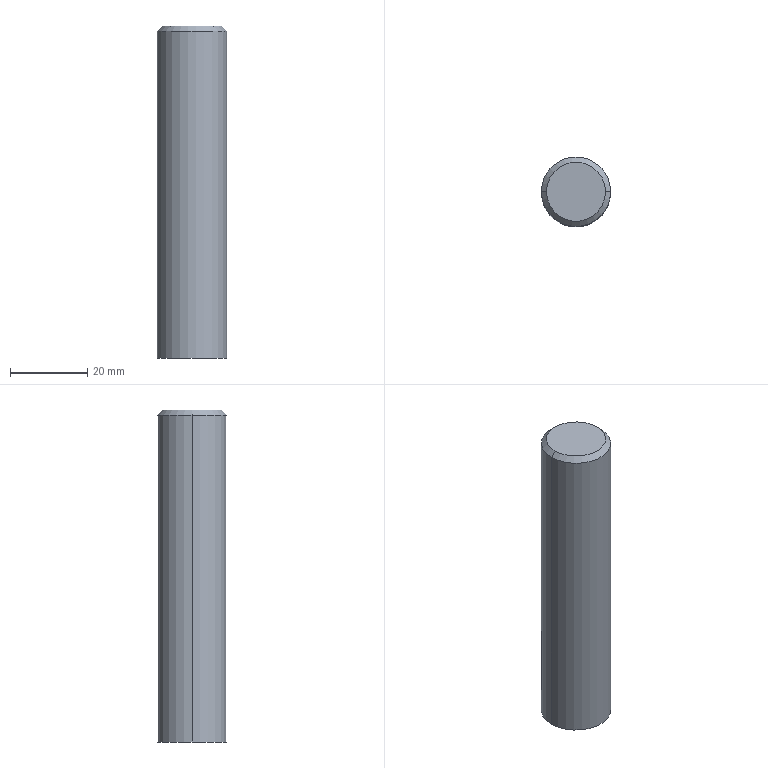Part | SolidWorks | features Extrusion 1, StudWizard 1 | 1 solid | 6 faces | box 18 x 18 x 86 mm | volume 21835 mm3 | cone 2 | cylinder 2 | plane 2 | commonest cylinder face diameters 18 x2
STEP:
#1=CARTESIAN_POINT('',(-7.647,0.,64.));
#2=VERTEX_POINT('',#1);
#3=CARTESIAN_POINT('',(7.647,0.,64.));
#4=VERTEX_POINT('',#3);
#5=CARTESIAN_POINT('',(0.,0.,64.));
#6=DIRECTION('',(0.,0.,-1.));
#7=DIRECTION('',(-1.,0.,0.));
#8=AXIS2_PLACEMENT_3D('',#5,#6,#7);
#9=CIRCLE('',#8,7.647);
#10=EDGE_CURVE('',#2,#4,#9,.T.);
#11=ORIENTED_EDGE('',*,*,#10,.T.);
#12=CARTESIAN_POINT('',(9.,0.,62.647));
#13=VERTEX_POINT('',#12);
#14=CARTESIAN_POINT('',(7.647,0.,64.));
#15=DIRECTION('',(0.7071,0.,-0.7071));
#16=VECTOR('',#15,1000.);
#17=LINE('',#14,#16);
#18=EDGE_CURVE('',#4,#13,#17,.T.);
#19=ORIENTED_EDGE('',*,*,#18,.T.);
#20=CARTESIAN_POINT('',(-9.,0.,62.647));
#21=VERTEX_POINT('',#20);
#22=CARTESIAN_POINT('',(0.,0.,62.647));
#23=DIRECTION('',(0.,0.,-1.));
#24=DIRECTION('',(-1.,0.,0.));
#25=AXIS2_PLACEMENT_3D('',#22,#23,#24);
#26=CIRCLE('',#25,9.);
#27=EDGE_CURVE('',#21,#13,#26,.T.);
#28=ORIENTED_EDGE('',*,*,#27,.F.);
#29=CARTESIAN_POINT('',(-7.647,0.,64.));
#30=DIRECTION('',(-0.7071,0.,-0.7071));
#31=VECTOR('',#30,1000.);
#32=LINE('',#29,#31);
#33=EDGE_CURVE('',#2,#21,#32,.T.);
#34=ORIENTED_EDGE('',*,*,#33,.F.);
#35=EDGE_LOOP('',(#11,#19,#28,#34));
#36=FACE_OUTER_BOUND('',#35,.T.);
#37=CARTESIAN_POINT('',(0.,0.,64.));
#38=DIRECTION('',(0.,0.,-1.));
#39=DIRECTION('',(-1.,0.,0.));
#40=AXIS2_PLACEMENT_3D('',#37,#38,#39);
#41=CONICAL_SURFACE('',#40,7.647,0.7854);
#42=ADVANCED_FACE('',(#36),#41,.T.);
#43=ORIENTED_EDGE('',*,*,#27,.T.);
#44=CARTESIAN_POINT('',(9.,0.,-22.));
#45=VERTEX_POINT('',#44);
#46=CARTESIAN_POINT('',(9.,0.,64.));
#47=DIRECTION('',(0.,0.,-1.));
#48=VECTOR('',#47,1000.);
#49=LINE('',#46,#48);
#50=EDGE_CURVE('',#13,#45,#49,.T.);
#51=ORIENTED_EDGE('',*,*,#50,.T.);
#52=CARTESIAN_POINT('',(-9.,0.,-22.));
#53=VERTEX_POINT('',#52);
#54=CARTESIAN_POINT('',(0.,0.,-22.));
#55=DIRECTION('',(0.,0.,-1.));
#56=DIRECTION('',(-1.,0.,0.));
#57=AXIS2_PLACEMENT_3D('',#54,#55,#56);
#58=CIRCLE('',#57,9.);
#59=EDGE_CURVE('',#53,#45,#58,.T.);
#60=ORIENTED_EDGE('',*,*,#59,.F.);
#61=CARTESIAN_POINT('',(-9.,0.,64.));
#62=DIRECTION('',(0.,0.,-1.));
#63=VECTOR('',#62,1000.);
#64=LINE('',#61,#63);
#65=EDGE_CURVE('',#21,#53,#64,.T.);
#66=ORIENTED_EDGE('',*,*,#65,.F.);
#67=EDGE_LOOP('',(#43,#51,#60,#66));
#68=FACE_OUTER_BOUND('',#67,.T.);
#69=CARTESIAN_POINT('',(0.,0.,64.));
#70=DIRECTION('',(0.,0.,-1.));
#71=DIRECTION('',(-1.,0.,0.));
#72=AXIS2_PLACEMENT_3D('',#69,#70,#71);
#73=CYLINDRICAL_SURFACE('',#72,9.);
#74=ADVANCED_FACE('',(#68),#73,.T.);
#75=ORIENTED_EDGE('',*,*,#10,.F.);
#76=CARTESIAN_POINT('',(0.,0.,64.));
#77=DIRECTION('',(0.,0.,-1.));
#78=DIRECTION('',(-1.,0.,0.));
#79=AXIS2_PLACEMENT_3D('',#76,#77,#78);
#80=CIRCLE('',#79,7.647);
#81=EDGE_CURVE('',#4,#2,#80,.T.);
#82=ORIENTED_EDGE('',*,*,#81,.F.);
#83=EDGE_LOOP('',(#75,#82));
#84=FACE_OUTER_BOUND('',#83,.T.);
#85=CARTESIAN_POINT('',(0.,0.,64.));
#86=DIRECTION('',(0.,0.,1.));
#87=DIRECTION('',(1.,0.,0.));
#88=AXIS2_PLACEMENT_3D('',#85,#86,#87);
#89=PLANE('',#88);
#90=ADVANCED_FACE('',(#84),#89,.T.);
#91=ORIENTED_EDGE('',*,*,#50,.F.);
#92=CARTESIAN_POINT('',(0.,0.,62.647));
#93=DIRECTION('',(0.,0.,-1.));
#94=DIRECTION('',(-1.,0.,0.));
#95=AXIS2_PLACEMENT_3D('',#92,#93,#94);
#96=CIRCLE('',#95,9.);
#97=EDGE_CURVE('',#13,#21,#96,.T.);
#98=ORIENTED_EDGE('',*,*,#97,.T.);
#99=ORIENTED_EDGE('',*,*,#65,.T.);
#100=CARTESIAN_POINT('',(0.,0.,-22.));
#101=DIRECTION('',(0.,0.,-1.));
#102=DIRECTION('',(-1.,0.,0.));
#103=AXIS2_PLACEMENT_3D('',#100,#101,#102);
#104=CIRCLE('',#103,9.);
#105=EDGE_CURVE('',#45,#53,#104,.T.);
#106=ORIENTED_EDGE('',*,*,#105,.F.);
#107=EDGE_LOOP('',(#91,#98,#99,#106));
#108=FACE_OUTER_BOUND('',#107,.T.);
#109=CARTESIAN_POINT('',(0.,0.,64.));
#110=DIRECTION('',(0.,0.,-1.));
#111=DIRECTION('',(-1.,0.,0.));
#112=AXIS2_PLACEMENT_3D('',#109,#110,#111);
#113=CYLINDRICAL_SURFACE('',#112,9.);
#114=ADVANCED_FACE('',(#108),#113,.T.);
#115=ORIENTED_EDGE('',*,*,#18,.F.);
#116=ORIENTED_EDGE('',*,*,#81,.T.);
#117=ORIENTED_EDGE('',*,*,#33,.T.);
#118=ORIENTED_EDGE('',*,*,#97,.F.);
#119=EDGE_LOOP('',(#115,#116,#117,#118));
#120=FACE_OUTER_BOUND('',#119,.T.);
#121=CARTESIAN_POINT('',(0.,0.,64.));
#122=DIRECTION('',(0.,0.,-1.));
#123=DIRECTION('',(-1.,0.,0.));
#124=AXIS2_PLACEMENT_3D('',#121,#122,#123);
#125=CONICAL_SURFACE('',#124,7.647,0.7854);
#126=ADVANCED_FACE('',(#120),#125,.T.);
#127=ORIENTED_EDGE('',*,*,#59,.T.);
#128=ORIENTED_EDGE('',*,*,#105,.T.);
#129=EDGE_LOOP('',(#127,#128));
#130=FACE_OUTER_BOUND('',#129,.T.);
#131=CARTESIAN_POINT('',(0.,0.,-22.));
#132=DIRECTION('',(0.,0.,1.));
#133=DIRECTION('',(1.,0.,0.));
#134=AXIS2_PLACEMENT_3D('',#131,#132,#133);
#135=PLANE('',#134);
#136=ADVANCED_FACE('',(#130),#135,.F.);
#137=CLOSED_SHELL('',(#42,#74,#90,#114,#126,#136));
#138=MANIFOLD_SOLID_BREP('',#137);
#139=CARTESIAN_POINT('',(0.,0.,0.));
#140=DIRECTION('',(0.,0.,1.));
#141=DIRECTION('',(1.,0.,0.));
#142=AXIS2_PLACEMENT_3D('',#139,#140,#141);
#143=(LENGTH_UNIT()NAMED_UNIT(*)SI_UNIT(.MILLI.,.METRE.));
#144=UNCERTAINTY_MEASURE_WITH_UNIT(LENGTH_MEASURE(0.00001),#143,'','');
#145=(NAMED_UNIT(*)PLANE_ANGLE_UNIT()SI_UNIT($,.RADIAN.));
#146=(NAMED_UNIT(*)SI_UNIT($,.STERADIAN.)SOLID_ANGLE_UNIT());
#147=(GEOMETRIC_REPRESENTATION_CONTEXT(3)GLOBAL_UNCERTAINTY_ASSIGNED_CONTEXT((#144))GLOBAL_UNIT_ASSIGNED_CONTEXT((#143,#145,#146))REPRESENTATION_CONTEXT('',''));
#148=ADVANCED_BREP_SHAPE_REPRESENTATION('',(#138,#142),#147);